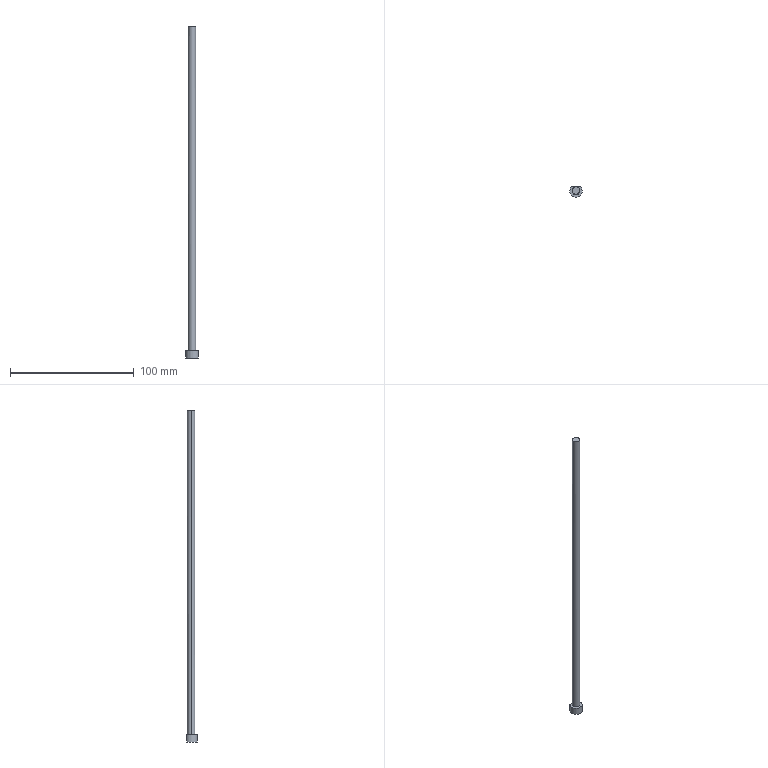Part | Creo | 1 solid | 7 faces | box 10 x 8.5 x 268.348 mm | volume 7845 mm3 | plane 4 | cylinder 3 | commonest cylinder face diameters 6 x2 10 x1
STEP:
#1=CARTESIAN_POINT('',(0.,0.,0.));
#2=DIRECTION('',(0.,0.,1.));
#3=DIRECTION('',(1.,0.,0.));
#4=AXIS2_PLACEMENT_3D('',#1,#2,#3);
#5=CARTESIAN_POINT('',(-4.87,-13.315,-332.441));
#6=VERTEX_POINT('',#5);
#7=CARTESIAN_POINT('',(-12.012,-13.315,-332.441));
#8=VERTEX_POINT('',#7);
#9=CARTESIAN_POINT('',(-4.87,-13.315,-332.441));
#10=DIRECTION('',(-1.,0.,0.));
#11=VECTOR('',#10,7.141);
#12=LINE('',#9,#11);
#13=EDGE_CURVE('',#6,#8,#12,.T.);
#14=ORIENTED_EDGE('',*,*,#13,.F.);
#15=CARTESIAN_POINT('',(-8.441,-16.815,-332.441));
#16=DIRECTION('',(0.,0.,-1.));
#17=DIRECTION('',(0.7141,0.7,0.));
#18=AXIS2_PLACEMENT_3D('',#15,#16,#17);
#19=CIRCLE('',#18,5.);
#20=EDGE_CURVE('',#6,#8,#19,.T.);
#21=ORIENTED_EDGE('',*,*,#20,.T.);
#22=EDGE_LOOP('',(#14,#21));
#23=FACE_OUTER_BOUND('',#22,.F.);
#24=CARTESIAN_POINT('',(-11.441,-16.815,-332.441));
#25=VERTEX_POINT('',#24);
#26=CARTESIAN_POINT('',(-5.441,-16.815,-332.441));
#27=VERTEX_POINT('',#26);
#28=CARTESIAN_POINT('',(-8.441,-16.815,-332.441));
#29=DIRECTION('',(0.,0.,-1.));
#30=DIRECTION('',(-1.,0.,0.));
#31=AXIS2_PLACEMENT_3D('',#28,#29,#30);
#32=CIRCLE('',#31,3.);
#33=EDGE_CURVE('',#25,#27,#32,.T.);
#34=ORIENTED_EDGE('',*,*,#33,.F.);
#35=CARTESIAN_POINT('',(-8.441,-16.815,-332.441));
#36=DIRECTION('',(0.,0.,-1.));
#37=DIRECTION('',(1.,0.,0.));
#38=AXIS2_PLACEMENT_3D('',#35,#36,#37);
#39=CIRCLE('',#38,3.);
#40=EDGE_CURVE('',#27,#25,#39,.T.);
#41=ORIENTED_EDGE('',*,*,#40,.F.);
#42=EDGE_LOOP('',(#34,#41));
#43=FACE_BOUND('',#42,.F.);
#44=CARTESIAN_POINT('',(-8.441,-16.815,-332.441));
#45=DIRECTION('',(0.,0.,-1.));
#46=DIRECTION('',(-1.,0.,0.));
#47=AXIS2_PLACEMENT_3D('',#44,#45,#46);
#48=PLANE('',#47);
#49=ADVANCED_FACE('',(#23,#43),#48,.F.);
#50=CARTESIAN_POINT('',(-5.441,-16.815,-70.101));
#51=VERTEX_POINT('',#50);
#52=CARTESIAN_POINT('',(-11.441,-16.814,-70.093));
#53=VERTEX_POINT('',#52);
#54=CARTESIAN_POINT('',(-5.441,-16.815,-70.101));
#55=CARTESIAN_POINT('',(-5.441,-16.486,-70.101));
#56=CARTESIAN_POINT('',(-5.543,-15.865,-70.101));
#57=CARTESIAN_POINT('',(-5.983,-15.009,-70.101));
#58=CARTESIAN_POINT('',(-6.659,-14.341,-70.1));
#59=CARTESIAN_POINT('',(-7.505,-13.913,-70.099));
#60=CARTESIAN_POINT('',(-8.439,-13.766,-70.097));
#61=CARTESIAN_POINT('',(-9.373,-13.912,-70.096));
#62=CARTESIAN_POINT('',(-10.22,-14.338,-70.095));
#63=CARTESIAN_POINT('',(-10.897,-15.006,-70.094));
#64=CARTESIAN_POINT('',(-11.337,-15.86,-70.094));
#65=CARTESIAN_POINT('',(-11.441,-16.485,-70.093));
#66=CARTESIAN_POINT('',(-11.441,-16.814,-70.093));
#67=B_SPLINE_CURVE_WITH_KNOTS('',3,(#54,#55,#56,#57,#58,#59,#60,#61,#62,#63,#64,#65,#66),.UNSPECIFIED.,.F.,.F.,(4,1,1,1,1,1,1,1,1,1,4),(0.,0.1,0.2,0.3,0.4,0.5,0.6,0.7,0.8,0.9,1.),.UNSPECIFIED.);
#68=EDGE_CURVE('',#51,#53,#67,.T.);
#69=ORIENTED_EDGE('',*,*,#68,.T.);
#70=CARTESIAN_POINT('',(-11.441,-16.815,-332.441));
#71=DIRECTION('',(0.000000004,0.00000521,1.));
#72=VECTOR('',#71,262.348);
#73=LINE('',#70,#72);
#74=EDGE_CURVE('',#25,#53,#73,.T.);
#75=ORIENTED_EDGE('',*,*,#74,.F.);
#76=ORIENTED_EDGE('',*,*,#33,.T.);
#77=CARTESIAN_POINT('',(-5.441,-16.815,-332.441));
#78=DIRECTION('',(0.,0.,1.));
#79=VECTOR('',#78,262.34);
#80=LINE('',#77,#79);
#81=EDGE_CURVE('',#27,#51,#80,.T.);
#82=ORIENTED_EDGE('',*,*,#81,.T.);
#83=EDGE_LOOP('',(#69,#75,#76,#82));
#84=FACE_OUTER_BOUND('',#83,.F.);
#85=CARTESIAN_POINT('',(-8.441,-16.815,-653.441));
#86=DIRECTION('',(0.,0.,1.));
#87=DIRECTION('',(1.,0.,0.));
#88=AXIS2_PLACEMENT_3D('',#85,#86,#87);
#89=CYLINDRICAL_SURFACE('',#88,3.);
#90=ADVANCED_FACE('',(#84),#89,.T.);
#91=CARTESIAN_POINT('',(-11.441,-16.814,-70.093));
#92=CARTESIAN_POINT('',(-11.441,-17.144,-70.093));
#93=CARTESIAN_POINT('',(-11.339,-17.762,-70.094));
#94=CARTESIAN_POINT('',(-10.9,-18.619,-70.094));
#95=CARTESIAN_POINT('',(-10.234,-19.279,-70.095));
#96=CARTESIAN_POINT('',(-9.395,-19.711,-70.096));
#97=CARTESIAN_POINT('',(-8.453,-19.865,-70.097));
#98=CARTESIAN_POINT('',(-7.511,-19.719,-70.099));
#99=CARTESIAN_POINT('',(-6.667,-19.294,-70.1));
#100=CARTESIAN_POINT('',(-5.989,-18.631,-70.101));
#101=CARTESIAN_POINT('',(-5.543,-17.765,-70.101));
#102=CARTESIAN_POINT('',(-5.441,-17.144,-70.101));
#103=CARTESIAN_POINT('',(-5.441,-16.815,-70.101));
#104=B_SPLINE_CURVE_WITH_KNOTS('',3,(#91,#92,#93,#94,#95,#96,#97,#98,#99,#100,#101,#102,#103),.UNSPECIFIED.,.F.,.F.,(4,1,1,1,1,1,1,1,1,1,4),(0.,0.1,0.2,0.3,0.4,0.5,0.6,0.7,0.8,0.9,1.),.UNSPECIFIED.);
#105=EDGE_CURVE('',#53,#51,#104,.T.);
#106=ORIENTED_EDGE('',*,*,#105,.F.);
#107=ORIENTED_EDGE('',*,*,#68,.F.);
#108=EDGE_LOOP('',(#106,#107));
#109=FACE_OUTER_BOUND('',#108,.F.);
#110=CARTESIAN_POINT('',(4.684,-7.032,-70.115));
#111=DIRECTION('',(-0.001312,0.000001793,-1.));
#112=DIRECTION('',(-1.,0.,0.001312));
#113=AXIS2_PLACEMENT_3D('',#110,#111,#112);
#114=PLANE('',#113);
#115=ADVANCED_FACE('',(#109),#114,.F.);
#116=ORIENTED_EDGE('',*,*,#105,.T.);
#117=ORIENTED_EDGE('',*,*,#81,.F.);
#118=ORIENTED_EDGE('',*,*,#40,.T.);
#119=ORIENTED_EDGE('',*,*,#74,.T.);
#120=EDGE_LOOP('',(#116,#117,#118,#119));
#121=FACE_OUTER_BOUND('',#120,.F.);
#122=CARTESIAN_POINT('',(-8.441,-16.815,-653.441));
#123=DIRECTION('',(0.,0.,1.));
#124=DIRECTION('',(1.,0.,0.));
#125=AXIS2_PLACEMENT_3D('',#122,#123,#124);
#126=CYLINDRICAL_SURFACE('',#125,3.);
#127=ADVANCED_FACE('',(#121),#126,.T.);
#128=CARTESIAN_POINT('',(-12.012,-13.315,-338.441));
#129=VERTEX_POINT('',#128);
#130=CARTESIAN_POINT('',(-12.012,-13.315,-332.441));
#131=DIRECTION('',(0.,0.,-1.));
#132=VECTOR('',#131,6.);
#133=LINE('',#130,#132);
#134=EDGE_CURVE('',#8,#129,#133,.T.);
#135=ORIENTED_EDGE('',*,*,#134,.T.);
#136=CARTESIAN_POINT('',(-4.87,-13.315,-338.441));
#137=VERTEX_POINT('',#136);
#138=CARTESIAN_POINT('',(-4.87,-13.315,-338.441));
#139=DIRECTION('',(-1.,0.,0.));
#140=VECTOR('',#139,7.141);
#141=LINE('',#138,#140);
#142=EDGE_CURVE('',#137,#129,#141,.T.);
#143=ORIENTED_EDGE('',*,*,#142,.F.);
#144=CARTESIAN_POINT('',(-4.87,-13.315,-338.441));
#145=DIRECTION('',(0.,0.,1.));
#146=VECTOR('',#145,6.);
#147=LINE('',#144,#146);
#148=EDGE_CURVE('',#137,#6,#147,.T.);
#149=ORIENTED_EDGE('',*,*,#148,.T.);
#150=ORIENTED_EDGE('',*,*,#13,.T.);
#151=EDGE_LOOP('',(#135,#143,#149,#150));
#152=FACE_OUTER_BOUND('',#151,.F.);
#153=CARTESIAN_POINT('',(-8.441,-13.315,-338.441));
#154=DIRECTION('',(0.,1.,0.));
#155=DIRECTION('',(0.,0.,1.));
#156=AXIS2_PLACEMENT_3D('',#153,#154,#155);
#157=PLANE('',#156);
#158=ADVANCED_FACE('',(#152),#157,.T.);
#159=CARTESIAN_POINT('',(-8.441,-16.815,-338.441));
#160=DIRECTION('',(0.,0.,1.));
#161=DIRECTION('',(-0.7141,0.7,0.));
#162=AXIS2_PLACEMENT_3D('',#159,#160,#161);
#163=CIRCLE('',#162,5.);
#164=EDGE_CURVE('',#129,#137,#163,.T.);
#165=ORIENTED_EDGE('',*,*,#164,.F.);
#166=ORIENTED_EDGE('',*,*,#134,.F.);
#167=ORIENTED_EDGE('',*,*,#20,.F.);
#168=ORIENTED_EDGE('',*,*,#148,.F.);
#169=EDGE_LOOP('',(#165,#166,#167,#168));
#170=FACE_OUTER_BOUND('',#169,.F.);
#171=CARTESIAN_POINT('',(-8.441,-16.815,-332.441));
#172=DIRECTION('',(0.,0.,-1.));
#173=DIRECTION('',(-1.,0.,0.));
#174=AXIS2_PLACEMENT_3D('',#171,#172,#173);
#175=CYLINDRICAL_SURFACE('',#174,5.);
#176=ADVANCED_FACE('',(#170),#175,.T.);
#177=ORIENTED_EDGE('',*,*,#164,.T.);
#178=ORIENTED_EDGE('',*,*,#142,.T.);
#179=EDGE_LOOP('',(#177,#178));
#180=FACE_OUTER_BOUND('',#179,.F.);
#181=CARTESIAN_POINT('',(-8.441,-16.815,-338.441));
#182=DIRECTION('',(0.,0.,-1.));
#183=DIRECTION('',(-1.,0.,0.));
#184=AXIS2_PLACEMENT_3D('',#181,#182,#183);
#185=PLANE('',#184);
#186=ADVANCED_FACE('',(#180),#185,.T.);
#187=CLOSED_SHELL('',(#49,#90,#115,#127,#158,#176,#186));
#188=MANIFOLD_SOLID_BREP('',#187);
#189=(LENGTH_UNIT()NAMED_UNIT(*)SI_UNIT(.MILLI.,.METRE.));
#190=UNCERTAINTY_MEASURE_WITH_UNIT(LENGTH_MEASURE(0.02687),#189,'','');
#191=(NAMED_UNIT(*)PLANE_ANGLE_UNIT()SI_UNIT($,.RADIAN.));
#192=PLANE_ANGLE_MEASURE_WITH_UNIT(PLANE_ANGLE_MEASURE(0.01745),#191);
#193=(CONVERSION_BASED_UNIT('DEGREE',#192)NAMED_UNIT(*)PLANE_ANGLE_UNIT());
#194=(NAMED_UNIT(*)SI_UNIT($,.STERADIAN.)SOLID_ANGLE_UNIT());
#195=(GEOMETRIC_REPRESENTATION_CONTEXT(3)GLOBAL_UNCERTAINTY_ASSIGNED_CONTEXT((#190))GLOBAL_UNIT_ASSIGNED_CONTEXT((#189,#193,#194))REPRESENTATION_CONTEXT('',''));
#196=ADVANCED_BREP_SHAPE_REPRESENTATION('',(#4,#188),#195);